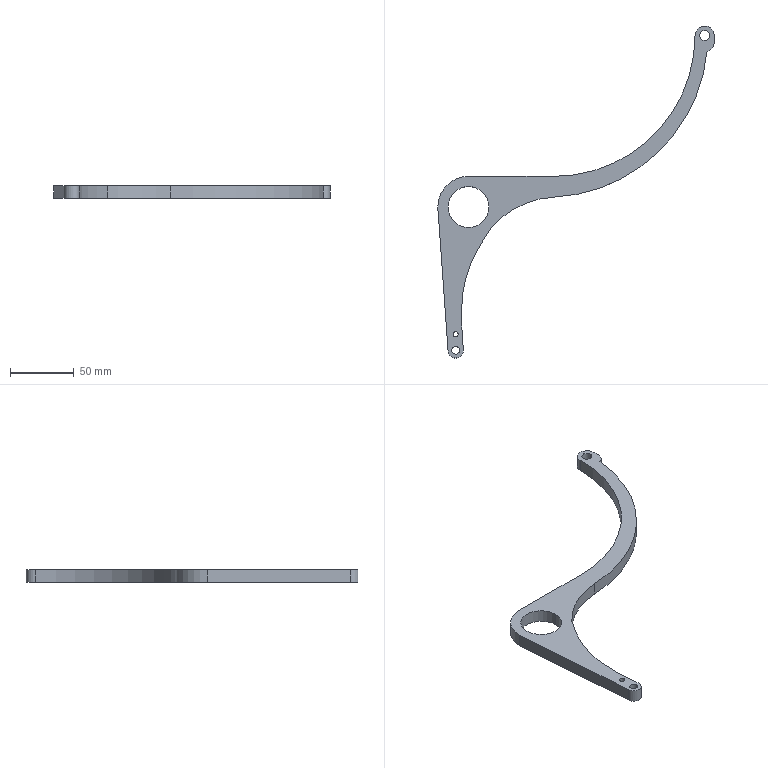Part | SolidWorks | features Extrusion 1 | 1 solid | 21 faces | box 216 x 259.5 x 10 mm | volume 61129 mm3 | cylinder 15 | plane 5 | spline 1 | commonest cylinder face diameters 4 x2 6 x2 7.838 x2 32 x2 12 x1 15 x1
STEP:
#1=CARTESIAN_POINT('',(-2.,12.5,10.));
#2=VERTEX_POINT('',#1);
#3=CARTESIAN_POINT('',(2.,12.5,10.));
#4=VERTEX_POINT('',#3);
#5=CARTESIAN_POINT('',(0.,12.5,10.));
#6=DIRECTION('',(0.,0.,1.));
#7=DIRECTION('',(1.,0.,0.));
#8=AXIS2_PLACEMENT_3D('',#5,#6,#7);
#9=CIRCLE('',#8,2.);
#10=EDGE_CURVE('',#2,#4,#9,.T.);
#11=ORIENTED_EDGE('',*,*,#10,.T.);
#12=CARTESIAN_POINT('',(2.,12.5,0.));
#13=VERTEX_POINT('',#12);
#14=CARTESIAN_POINT('',(2.,12.5,10.));
#15=DIRECTION('',(0.,0.,-1.));
#16=VECTOR('',#15,1000.);
#17=LINE('',#14,#16);
#18=EDGE_CURVE('',#4,#13,#17,.T.);
#19=ORIENTED_EDGE('',*,*,#18,.T.);
#20=CARTESIAN_POINT('',(-2.,12.5,0.));
#21=VERTEX_POINT('',#20);
#22=CARTESIAN_POINT('',(0.,12.5,0.));
#23=DIRECTION('',(0.,0.,1.));
#24=DIRECTION('',(1.,0.,0.));
#25=AXIS2_PLACEMENT_3D('',#22,#23,#24);
#26=CIRCLE('',#25,2.);
#27=EDGE_CURVE('',#21,#13,#26,.T.);
#28=ORIENTED_EDGE('',*,*,#27,.F.);
#29=CARTESIAN_POINT('',(-2.,12.5,10.));
#30=DIRECTION('',(0.,0.,-1.));
#31=VECTOR('',#30,1000.);
#32=LINE('',#29,#31);
#33=EDGE_CURVE('',#2,#21,#32,.T.);
#34=ORIENTED_EDGE('',*,*,#33,.F.);
#35=EDGE_LOOP('',(#11,#19,#28,#34));
#36=FACE_OUTER_BOUND('',#35,.T.);
#37=CARTESIAN_POINT('',(0.,12.5,10.));
#38=DIRECTION('',(0.,0.,-1.));
#39=DIRECTION('',(-1.,0.,0.));
#40=AXIS2_PLACEMENT_3D('',#37,#38,#39);
#41=CYLINDRICAL_SURFACE('',#40,2.);
#42=ADVANCED_FACE('',(#36),#41,.F.);
#43=CARTESIAN_POINT('',(190.581,246.,10.));
#44=VERTEX_POINT('',#43);
#45=CARTESIAN_POINT('',(198.419,246.,10.));
#46=VERTEX_POINT('',#45);
#47=CARTESIAN_POINT('',(194.5,246.,10.));
#48=DIRECTION('',(0.,0.,1.));
#49=DIRECTION('',(1.,0.,0.));
#50=AXIS2_PLACEMENT_3D('',#47,#48,#49);
#51=CIRCLE('',#50,3.919);
#52=EDGE_CURVE('',#44,#46,#51,.T.);
#53=ORIENTED_EDGE('',*,*,#52,.T.);
#54=CARTESIAN_POINT('',(198.419,246.,0.));
#55=VERTEX_POINT('',#54);
#56=CARTESIAN_POINT('',(198.419,246.,10.));
#57=DIRECTION('',(0.,0.,-1.));
#58=VECTOR('',#57,1000.);
#59=LINE('',#56,#58);
#60=EDGE_CURVE('',#46,#55,#59,.T.);
#61=ORIENTED_EDGE('',*,*,#60,.T.);
#62=CARTESIAN_POINT('',(190.581,246.,0.));
#63=VERTEX_POINT('',#62);
#64=CARTESIAN_POINT('',(194.5,246.,0.));
#65=DIRECTION('',(0.,0.,1.));
#66=DIRECTION('',(1.,0.,0.));
#67=AXIS2_PLACEMENT_3D('',#64,#65,#66);
#68=CIRCLE('',#67,3.919);
#69=EDGE_CURVE('',#63,#55,#68,.T.);
#70=ORIENTED_EDGE('',*,*,#69,.F.);
#71=CARTESIAN_POINT('',(190.581,246.,10.));
#72=DIRECTION('',(0.,0.,-1.));
#73=VECTOR('',#72,1000.);
#74=LINE('',#71,#73);
#75=EDGE_CURVE('',#44,#63,#74,.T.);
#76=ORIENTED_EDGE('',*,*,#75,.F.);
#77=EDGE_LOOP('',(#53,#61,#70,#76));
#78=FACE_OUTER_BOUND('',#77,.T.);
#79=CARTESIAN_POINT('',(194.5,246.,10.));
#80=DIRECTION('',(0.,0.,-1.));
#81=DIRECTION('',(-1.,0.,0.));
#82=AXIS2_PLACEMENT_3D('',#79,#80,#81);
#83=CYLINDRICAL_SURFACE('',#82,3.919);
#84=ADVANCED_FACE('',(#78),#83,.F.);
#85=CARTESIAN_POINT('',(-6.,112.,10.));
#86=VERTEX_POINT('',#85);
#87=CARTESIAN_POINT('',(26.,112.,10.));
#88=VERTEX_POINT('',#87);
#89=CARTESIAN_POINT('',(10.,112.,10.));
#90=DIRECTION('',(0.,0.,1.));
#91=DIRECTION('',(1.,0.,0.));
#92=AXIS2_PLACEMENT_3D('',#89,#90,#91);
#93=CIRCLE('',#92,16.);
#94=EDGE_CURVE('',#86,#88,#93,.T.);
#95=ORIENTED_EDGE('',*,*,#94,.T.);
#96=CARTESIAN_POINT('',(26.,112.,0.));
#97=VERTEX_POINT('',#96);
#98=CARTESIAN_POINT('',(26.,112.,10.));
#99=DIRECTION('',(0.,0.,-1.));
#100=VECTOR('',#99,1000.);
#101=LINE('',#98,#100);
#102=EDGE_CURVE('',#88,#97,#101,.T.);
#103=ORIENTED_EDGE('',*,*,#102,.T.);
#104=CARTESIAN_POINT('',(-6.,112.,0.));
#105=VERTEX_POINT('',#104);
#106=CARTESIAN_POINT('',(10.,112.,0.));
#107=DIRECTION('',(0.,0.,1.));
#108=DIRECTION('',(1.,0.,0.));
#109=AXIS2_PLACEMENT_3D('',#106,#107,#108);
#110=CIRCLE('',#109,16.);
#111=EDGE_CURVE('',#105,#97,#110,.T.);
#112=ORIENTED_EDGE('',*,*,#111,.F.);
#113=CARTESIAN_POINT('',(-6.,112.,10.));
#114=DIRECTION('',(0.,0.,-1.));
#115=VECTOR('',#114,1000.);
#116=LINE('',#113,#115);
#117=EDGE_CURVE('',#86,#105,#116,.T.);
#118=ORIENTED_EDGE('',*,*,#117,.F.);
#119=EDGE_LOOP('',(#95,#103,#112,#118));
#120=FACE_OUTER_BOUND('',#119,.T.);
#121=CARTESIAN_POINT('',(10.,112.,10.));
#122=DIRECTION('',(0.,0.,-1.));
#123=DIRECTION('',(-1.,0.,0.));
#124=AXIS2_PLACEMENT_3D('',#121,#122,#123);
#125=CYLINDRICAL_SURFACE('',#124,16.);
#126=ADVANCED_FACE('',(#120),#125,.F.);
#127=CARTESIAN_POINT('',(-3.,0.,10.));
#128=VERTEX_POINT('',#127);
#129=CARTESIAN_POINT('',(3.,0.,10.));
#130=VERTEX_POINT('',#129);
#131=CARTESIAN_POINT('',(0.,0.,10.));
#132=DIRECTION('',(0.,0.,1.));
#133=DIRECTION('',(1.,0.,0.));
#134=AXIS2_PLACEMENT_3D('',#131,#132,#133);
#135=CIRCLE('',#134,3.);
#136=EDGE_CURVE('',#128,#130,#135,.T.);
#137=ORIENTED_EDGE('',*,*,#136,.T.);
#138=CARTESIAN_POINT('',(3.,0.,0.));
#139=VERTEX_POINT('',#138);
#140=CARTESIAN_POINT('',(3.,0.,10.));
#141=DIRECTION('',(0.,0.,-1.));
#142=VECTOR('',#141,1000.);
#143=LINE('',#140,#142);
#144=EDGE_CURVE('',#130,#139,#143,.T.);
#145=ORIENTED_EDGE('',*,*,#144,.T.);
#146=CARTESIAN_POINT('',(-3.,0.,0.));
#147=VERTEX_POINT('',#146);
#148=CARTESIAN_POINT('',(0.,0.,0.));
#149=DIRECTION('',(0.,0.,1.));
#150=DIRECTION('',(1.,0.,0.));
#151=AXIS2_PLACEMENT_3D('',#148,#149,#150);
#152=CIRCLE('',#151,3.);
#153=EDGE_CURVE('',#147,#139,#152,.T.);
#154=ORIENTED_EDGE('',*,*,#153,.F.);
#155=CARTESIAN_POINT('',(-3.,0.,10.));
#156=DIRECTION('',(0.,0.,-1.));
#157=VECTOR('',#156,1000.);
#158=LINE('',#155,#157);
#159=EDGE_CURVE('',#128,#147,#158,.T.);
#160=ORIENTED_EDGE('',*,*,#159,.F.);
#161=EDGE_LOOP('',(#137,#145,#154,#160));
#162=FACE_OUTER_BOUND('',#161,.T.);
#163=CARTESIAN_POINT('',(0.,0.,10.));
#164=DIRECTION('',(0.,0.,-1.));
#165=DIRECTION('',(-1.,0.,0.));
#166=AXIS2_PLACEMENT_3D('',#163,#164,#165);
#167=CYLINDRICAL_SURFACE('',#166,3.);
#168=ADVANCED_FACE('',(#162),#167,.F.);
#169=ORIENTED_EDGE('',*,*,#52,.F.);
#170=CARTESIAN_POINT('',(194.5,246.,10.));
#171=DIRECTION('',(0.,0.,1.));
#172=DIRECTION('',(1.,0.,0.));
#173=AXIS2_PLACEMENT_3D('',#170,#171,#172);
#174=CIRCLE('',#173,3.919);
#175=EDGE_CURVE('',#46,#44,#174,.T.);
#176=ORIENTED_EDGE('',*,*,#175,.F.);
#177=EDGE_LOOP('',(#169,#176));
#178=FACE_BOUND('',#177,.T.);
#179=ORIENTED_EDGE('',*,*,#136,.F.);
#180=CARTESIAN_POINT('',(0.,0.,10.));
#181=DIRECTION('',(0.,0.,1.));
#182=DIRECTION('',(1.,0.,0.));
#183=AXIS2_PLACEMENT_3D('',#180,#181,#182);
#184=CIRCLE('',#183,3.);
#185=EDGE_CURVE('',#130,#128,#184,.T.);
#186=ORIENTED_EDGE('',*,*,#185,.F.);
#187=EDGE_LOOP('',(#179,#186));
#188=FACE_BOUND('',#187,.T.);
#189=CARTESIAN_POINT('',(10.,136.,10.));
#190=VERTEX_POINT('',#189);
#191=CARTESIAN_POINT('',(-14.,112.,10.));
#192=VERTEX_POINT('',#191);
#193=CARTESIAN_POINT('',(10.,112.,10.));
#194=DIRECTION('',(0.,0.,1.));
#195=DIRECTION('',(1.,0.,0.));
#196=AXIS2_PLACEMENT_3D('',#193,#194,#195);
#197=CIRCLE('',#196,24.);
#198=EDGE_CURVE('',#190,#192,#197,.T.);
#199=ORIENTED_EDGE('',*,*,#198,.T.);
#200=CARTESIAN_POINT('',(-6.,0.,10.));
#201=VERTEX_POINT('',#200);
#202=CARTESIAN_POINT('',(-14.,112.,10.));
#203=DIRECTION('',(0.07125,-0.9975,0.));
#204=VECTOR('',#203,1000.);
#205=LINE('',#202,#204);
#206=EDGE_CURVE('',#192,#201,#205,.T.);
#207=ORIENTED_EDGE('',*,*,#206,.T.);
#208=CARTESIAN_POINT('',(6.,0.,10.));
#209=VERTEX_POINT('',#208);
#210=CARTESIAN_POINT('',(0.,0.,10.));
#211=DIRECTION('',(0.,0.,1.));
#212=DIRECTION('',(1.,0.,0.));
#213=AXIS2_PLACEMENT_3D('',#210,#211,#212);
#214=CIRCLE('',#213,6.);
#215=EDGE_CURVE('',#201,#209,#214,.T.);
#216=ORIENTED_EDGE('',*,*,#215,.T.);
#217=CARTESIAN_POINT('',(28.005,96.131,10.));
#218=VERTEX_POINT('',#217);
#219=CARTESIAN_POINT('',(6.,0.,10.));
#220=CARTESIAN_POINT('',(1.589,45.681,10.));
#221=CARTESIAN_POINT('',(5.604,63.643,10.));
#222=CARTESIAN_POINT('',(28.005,96.131,10.));
#223=B_SPLINE_CURVE_WITH_KNOTS('',3,(#219,#220,#221,#222),.UNSPECIFIED.,.F.,.F.,(4,4),(0.,0.7882),.UNSPECIFIED.);
#224=EDGE_CURVE('',#209,#218,#223,.T.);
#225=ORIENTED_EDGE('',*,*,#224,.T.);
#226=CARTESIAN_POINT('',(77.,119.767,10.));
#227=VERTEX_POINT('',#226);
#228=CARTESIAN_POINT('',(80.543,49.825,10.));
#229=DIRECTION('',(0.,0.,-1.));
#230=DIRECTION('',(1.,0.,0.));
#231=AXIS2_PLACEMENT_3D('',#228,#229,#230);
#232=CIRCLE('',#231,70.032);
#233=EDGE_CURVE('',#218,#227,#232,.T.);
#234=ORIENTED_EDGE('',*,*,#233,.T.);
#235=CARTESIAN_POINT('',(196.38,233.495,10.));
#236=VERTEX_POINT('',#235);
#237=CARTESIAN_POINT('',(70.606,246.,10.));
#238=DIRECTION('',(0.,0.,1.));
#239=DIRECTION('',(1.,0.,0.));
#240=AXIS2_PLACEMENT_3D('',#237,#238,#239);
#241=CIRCLE('',#240,126.394);
#242=EDGE_CURVE('',#227,#236,#241,.T.);
#243=ORIENTED_EDGE('',*,*,#242,.T.);
#244=CARTESIAN_POINT('',(202.,241.,10.));
#245=VERTEX_POINT('',#244);
#246=CARTESIAN_POINT('',(194.179,241.,10.));
#247=DIRECTION('',(0.,0.,1.));
#248=DIRECTION('',(1.,0.,0.));
#249=AXIS2_PLACEMENT_3D('',#246,#247,#248);
#250=CIRCLE('',#249,7.821);
#251=EDGE_CURVE('',#236,#245,#250,.T.);
#252=ORIENTED_EDGE('',*,*,#251,.T.);
#253=CARTESIAN_POINT('',(202.,246.,10.));
#254=VERTEX_POINT('',#253);
#255=CARTESIAN_POINT('',(202.,246.,10.));
#256=DIRECTION('',(0.,1.,0.));
#257=VECTOR('',#256,1000.);
#258=LINE('',#255,#257);
#259=EDGE_CURVE('',#245,#254,#258,.T.);
#260=ORIENTED_EDGE('',*,*,#259,.T.);
#261=CARTESIAN_POINT('',(187.,246.,10.));
#262=VERTEX_POINT('',#261);
#263=CARTESIAN_POINT('',(194.5,246.,10.));
#264=DIRECTION('',(0.,0.,1.));
#265=DIRECTION('',(1.,0.,0.));
#266=AXIS2_PLACEMENT_3D('',#263,#264,#265);
#267=CIRCLE('',#266,7.5);
#268=EDGE_CURVE('',#254,#262,#267,.T.);
#269=ORIENTED_EDGE('',*,*,#268,.T.);
#270=CARTESIAN_POINT('',(77.,136.,10.));
#271=VERTEX_POINT('',#270);
#272=CARTESIAN_POINT('',(77.,246.,10.));
#273=DIRECTION('',(0.,0.,-1.));
#274=DIRECTION('',(1.,0.,0.));
#275=AXIS2_PLACEMENT_3D('',#272,#273,#274);
#276=CIRCLE('',#275,110.);
#277=EDGE_CURVE('',#262,#271,#276,.T.);
#278=ORIENTED_EDGE('',*,*,#277,.T.);
#279=CARTESIAN_POINT('',(10.,136.,10.));
#280=DIRECTION('',(-1.,0.,0.));
#281=VECTOR('',#280,1000.);
#282=LINE('',#279,#281);
#283=EDGE_CURVE('',#271,#190,#282,.T.);
#284=ORIENTED_EDGE('',*,*,#283,.T.);
#285=EDGE_LOOP('',(#199,#207,#216,#225,#234,#243,#252,#260,#269,#278,#284));
#286=FACE_OUTER_BOUND('',#285,.T.);
#287=ORIENTED_EDGE('',*,*,#94,.F.);
#288=CARTESIAN_POINT('',(10.,112.,10.));
#289=DIRECTION('',(0.,0.,1.));
#290=DIRECTION('',(1.,0.,0.));
#291=AXIS2_PLACEMENT_3D('',#288,#289,#290);
#292=CIRCLE('',#291,16.);
#293=EDGE_CURVE('',#88,#86,#292,.T.);
#294=ORIENTED_EDGE('',*,*,#293,.F.);
#295=EDGE_LOOP('',(#287,#294));
#296=FACE_BOUND('',#295,.T.);
#297=ORIENTED_EDGE('',*,*,#10,.F.);
#298=CARTESIAN_POINT('',(0.,12.5,10.));
#299=DIRECTION('',(0.,0.,1.));
#300=DIRECTION('',(1.,0.,0.));
#301=AXIS2_PLACEMENT_3D('',#298,#299,#300);
#302=CIRCLE('',#301,2.);
#303=EDGE_CURVE('',#4,#2,#302,.T.);
#304=ORIENTED_EDGE('',*,*,#303,.F.);
#305=EDGE_LOOP('',(#297,#304));
#306=FACE_BOUND('',#305,.T.);
#307=CARTESIAN_POINT('',(10.,112.,10.));
#308=DIRECTION('',(0.,0.,1.));
#309=DIRECTION('',(1.,0.,0.));
#310=AXIS2_PLACEMENT_3D('',#307,#308,#309);
#311=PLANE('',#310);
#312=ADVANCED_FACE('',(#178,#188,#286,#296,#306),#311,.T.);
#313=CARTESIAN_POINT('',(10.,136.,0.));
#314=VERTEX_POINT('',#313);
#315=CARTESIAN_POINT('',(-14.,112.,0.));
#316=VERTEX_POINT('',#315);
#317=CARTESIAN_POINT('',(10.,112.,0.));
#318=DIRECTION('',(0.,0.,1.));
#319=DIRECTION('',(1.,0.,0.));
#320=AXIS2_PLACEMENT_3D('',#317,#318,#319);
#321=CIRCLE('',#320,24.);
#322=EDGE_CURVE('',#314,#316,#321,.T.);
#323=ORIENTED_EDGE('',*,*,#322,.F.);
#324=CARTESIAN_POINT('',(77.,136.,0.));
#325=VERTEX_POINT('',#324);
#326=CARTESIAN_POINT('',(10.,136.,0.));
#327=DIRECTION('',(-1.,0.,0.));
#328=VECTOR('',#327,1000.);
#329=LINE('',#326,#328);
#330=EDGE_CURVE('',#325,#314,#329,.T.);
#331=ORIENTED_EDGE('',*,*,#330,.F.);
#332=CARTESIAN_POINT('',(187.,246.,0.));
#333=VERTEX_POINT('',#332);
#334=CARTESIAN_POINT('',(77.,246.,0.));
#335=DIRECTION('',(0.,0.,-1.));
#336=DIRECTION('',(1.,0.,0.));
#337=AXIS2_PLACEMENT_3D('',#334,#335,#336);
#338=CIRCLE('',#337,110.);
#339=EDGE_CURVE('',#333,#325,#338,.T.);
#340=ORIENTED_EDGE('',*,*,#339,.F.);
#341=CARTESIAN_POINT('',(202.,246.,0.));
#342=VERTEX_POINT('',#341);
#343=CARTESIAN_POINT('',(194.5,246.,0.));
#344=DIRECTION('',(0.,0.,1.));
#345=DIRECTION('',(1.,0.,0.));
#346=AXIS2_PLACEMENT_3D('',#343,#344,#345);
#347=CIRCLE('',#346,7.5);
#348=EDGE_CURVE('',#342,#333,#347,.T.);
#349=ORIENTED_EDGE('',*,*,#348,.F.);
#350=CARTESIAN_POINT('',(202.,241.,0.));
#351=VERTEX_POINT('',#350);
#352=CARTESIAN_POINT('',(202.,246.,0.));
#353=DIRECTION('',(0.,1.,0.));
#354=VECTOR('',#353,1000.);
#355=LINE('',#352,#354);
#356=EDGE_CURVE('',#351,#342,#355,.T.);
#357=ORIENTED_EDGE('',*,*,#356,.F.);
#358=CARTESIAN_POINT('',(196.38,233.495,0.));
#359=VERTEX_POINT('',#358);
#360=CARTESIAN_POINT('',(194.179,241.,0.));
#361=DIRECTION('',(0.,0.,1.));
#362=DIRECTION('',(1.,0.,0.));
#363=AXIS2_PLACEMENT_3D('',#360,#361,#362);
#364=CIRCLE('',#363,7.821);
#365=EDGE_CURVE('',#359,#351,#364,.T.);
#366=ORIENTED_EDGE('',*,*,#365,.F.);
#367=CARTESIAN_POINT('',(77.,119.767,0.));
#368=VERTEX_POINT('',#367);
#369=CARTESIAN_POINT('',(70.606,246.,0.));
#370=DIRECTION('',(0.,0.,1.));
#371=DIRECTION('',(1.,0.,0.));
#372=AXIS2_PLACEMENT_3D('',#369,#370,#371);
#373=CIRCLE('',#372,126.394);
#374=EDGE_CURVE('',#368,#359,#373,.T.);
#375=ORIENTED_EDGE('',*,*,#374,.F.);
#376=CARTESIAN_POINT('',(28.005,96.131,0.));
#377=VERTEX_POINT('',#376);
#378=CARTESIAN_POINT('',(80.543,49.825,0.));
#379=DIRECTION('',(0.,0.,-1.));
#380=DIRECTION('',(1.,0.,0.));
#381=AXIS2_PLACEMENT_3D('',#378,#379,#380);
#382=CIRCLE('',#381,70.032);
#383=EDGE_CURVE('',#377,#368,#382,.T.);
#384=ORIENTED_EDGE('',*,*,#383,.F.);
#385=CARTESIAN_POINT('',(6.,0.,0.));
#386=VERTEX_POINT('',#385);
#387=CARTESIAN_POINT('',(6.,0.,0.));
#388=CARTESIAN_POINT('',(1.589,45.681,0.));
#389=CARTESIAN_POINT('',(5.604,63.643,0.));
#390=CARTESIAN_POINT('',(28.005,96.131,0.));
#391=B_SPLINE_CURVE_WITH_KNOTS('',3,(#387,#388,#389,#390),.UNSPECIFIED.,.F.,.F.,(4,4),(0.,0.7882),.UNSPECIFIED.);
#392=EDGE_CURVE('',#386,#377,#391,.T.);
#393=ORIENTED_EDGE('',*,*,#392,.F.);
#394=CARTESIAN_POINT('',(-6.,0.,0.));
#395=VERTEX_POINT('',#394);
#396=CARTESIAN_POINT('',(0.,0.,0.));
#397=DIRECTION('',(0.,0.,1.));
#398=DIRECTION('',(1.,0.,0.));
#399=AXIS2_PLACEMENT_3D('',#396,#397,#398);
#400=CIRCLE('',#399,6.);
#401=EDGE_CURVE('',#395,#386,#400,.T.);
#402=ORIENTED_EDGE('',*,*,#401,.F.);
#403=CARTESIAN_POINT('',(-14.,112.,0.));
#404=DIRECTION('',(0.07125,-0.9975,0.));
#405=VECTOR('',#404,1000.);
#406=LINE('',#403,#405);
#407=EDGE_CURVE('',#316,#395,#406,.T.);
#408=ORIENTED_EDGE('',*,*,#407,.F.);
#409=EDGE_LOOP('',(#323,#331,#340,#349,#357,#366,#375,#384,#393,#402,#408));
#410=FACE_OUTER_BOUND('',#409,.T.);
#411=ORIENTED_EDGE('',*,*,#153,.T.);
#412=CARTESIAN_POINT('',(0.,0.,0.));
#413=DIRECTION('',(0.,0.,1.));
#414=DIRECTION('',(1.,0.,0.));
#415=AXIS2_PLACEMENT_3D('',#412,#413,#414);
#416=CIRCLE('',#415,3.);
#417=EDGE_CURVE('',#139,#147,#416,.T.);
#418=ORIENTED_EDGE('',*,*,#417,.T.);
#419=EDGE_LOOP('',(#411,#418));
#420=FACE_BOUND('',#419,.T.);
#421=ORIENTED_EDGE('',*,*,#111,.T.);
#422=CARTESIAN_POINT('',(10.,112.,0.));
#423=DIRECTION('',(0.,0.,1.));
#424=DIRECTION('',(1.,0.,0.));
#425=AXIS2_PLACEMENT_3D('',#422,#423,#424);
#426=CIRCLE('',#425,16.);
#427=EDGE_CURVE('',#97,#105,#426,.T.);
#428=ORIENTED_EDGE('',*,*,#427,.T.);
#429=EDGE_LOOP('',(#421,#428));
#430=FACE_BOUND('',#429,.T.);
#431=ORIENTED_EDGE('',*,*,#69,.T.);
#432=CARTESIAN_POINT('',(194.5,246.,0.));
#433=DIRECTION('',(0.,0.,1.));
#434=DIRECTION('',(1.,0.,0.));
#435=AXIS2_PLACEMENT_3D('',#432,#433,#434);
#436=CIRCLE('',#435,3.919);
#437=EDGE_CURVE('',#55,#63,#436,.T.);
#438=ORIENTED_EDGE('',*,*,#437,.T.);
#439=EDGE_LOOP('',(#431,#438));
#440=FACE_BOUND('',#439,.T.);
#441=ORIENTED_EDGE('',*,*,#27,.T.);
#442=CARTESIAN_POINT('',(0.,12.5,0.));
#443=DIRECTION('',(0.,0.,1.));
#444=DIRECTION('',(1.,0.,0.));
#445=AXIS2_PLACEMENT_3D('',#442,#443,#444);
#446=CIRCLE('',#445,2.);
#447=EDGE_CURVE('',#13,#21,#446,.T.);
#448=ORIENTED_EDGE('',*,*,#447,.T.);
#449=EDGE_LOOP('',(#441,#448));
#450=FACE_BOUND('',#449,.T.);
#451=CARTESIAN_POINT('',(10.,112.,0.));
#452=DIRECTION('',(0.,0.,1.));
#453=DIRECTION('',(1.,0.,0.));
#454=AXIS2_PLACEMENT_3D('',#451,#452,#453);
#455=PLANE('',#454);
#456=ADVANCED_FACE('',(#410,#420,#430,#440,#450),#455,.F.);
#457=ORIENTED_EDGE('',*,*,#322,.T.);
#458=CARTESIAN_POINT('',(-14.,112.,10.));
#459=DIRECTION('',(0.,0.,-1.));
#460=VECTOR('',#459,1000.);
#461=LINE('',#458,#460);
#462=EDGE_CURVE('',#192,#316,#461,.T.);
#463=ORIENTED_EDGE('',*,*,#462,.F.);
#464=ORIENTED_EDGE('',*,*,#198,.F.);
#465=CARTESIAN_POINT('',(10.,136.,10.));
#466=DIRECTION('',(0.,0.,-1.));
#467=VECTOR('',#466,1000.);
#468=LINE('',#465,#467);
#469=EDGE_CURVE('',#190,#314,#468,.T.);
#470=ORIENTED_EDGE('',*,*,#469,.T.);
#471=EDGE_LOOP('',(#457,#463,#464,#470));
#472=FACE_OUTER_BOUND('',#471,.T.);
#473=CARTESIAN_POINT('',(10.,112.,10.));
#474=DIRECTION('',(0.,0.,-1.));
#475=DIRECTION('',(-1.,0.,0.));
#476=AXIS2_PLACEMENT_3D('',#473,#474,#475);
#477=CYLINDRICAL_SURFACE('',#476,24.);
#478=ADVANCED_FACE('',(#472),#477,.T.);
#479=ORIENTED_EDGE('',*,*,#407,.T.);
#480=CARTESIAN_POINT('',(-6.,0.,10.));
#481=DIRECTION('',(0.,0.,-1.));
#482=VECTOR('',#481,1000.);
#483=LINE('',#480,#482);
#484=EDGE_CURVE('',#201,#395,#483,.T.);
#485=ORIENTED_EDGE('',*,*,#484,.F.);
#486=ORIENTED_EDGE('',*,*,#206,.F.);
#487=ORIENTED_EDGE('',*,*,#462,.T.);
#488=EDGE_LOOP('',(#479,#485,#486,#487));
#489=FACE_OUTER_BOUND('',#488,.T.);
#490=CARTESIAN_POINT('',(-14.,112.,10.));
#491=DIRECTION('',(0.9975,0.07125,0.));
#492=DIRECTION('',(-0.07125,0.9975,0.));
#493=AXIS2_PLACEMENT_3D('',#490,#491,#492);
#494=PLANE('',#493);
#495=ADVANCED_FACE('',(#489),#494,.F.);
#496=ORIENTED_EDGE('',*,*,#401,.T.);
#497=CARTESIAN_POINT('',(6.,0.,10.));
#498=DIRECTION('',(0.,0.,-1.));
#499=VECTOR('',#498,1000.);
#500=LINE('',#497,#499);
#501=EDGE_CURVE('',#209,#386,#500,.T.);
#502=ORIENTED_EDGE('',*,*,#501,.F.);
#503=ORIENTED_EDGE('',*,*,#215,.F.);
#504=ORIENTED_EDGE('',*,*,#484,.T.);
#505=EDGE_LOOP('',(#496,#502,#503,#504));
#506=FACE_OUTER_BOUND('',#505,.T.);
#507=CARTESIAN_POINT('',(0.,0.,10.));
#508=DIRECTION('',(0.,0.,-1.));
#509=DIRECTION('',(-1.,0.,0.));
#510=AXIS2_PLACEMENT_3D('',#507,#508,#509);
#511=CYLINDRICAL_SURFACE('',#510,6.);
#512=ADVANCED_FACE('',(#506),#511,.T.);
#513=ORIENTED_EDGE('',*,*,#392,.T.);
#514=CARTESIAN_POINT('',(28.005,96.131,10.));
#515=DIRECTION('',(0.,0.,-1.));
#516=VECTOR('',#515,1000.);
#517=LINE('',#514,#516);
#518=EDGE_CURVE('',#218,#377,#517,.T.);
#519=ORIENTED_EDGE('',*,*,#518,.F.);
#520=ORIENTED_EDGE('',*,*,#224,.F.);
#521=ORIENTED_EDGE('',*,*,#501,.T.);
#522=EDGE_LOOP('',(#513,#519,#520,#521));
#523=FACE_OUTER_BOUND('',#522,.T.);
#524=CARTESIAN_POINT('',(6.,0.,10.));
#525=CARTESIAN_POINT('',(6.,0.,0.));
#526=CARTESIAN_POINT('',(1.589,45.681,10.));
#527=CARTESIAN_POINT('',(1.589,45.681,0.));
#528=CARTESIAN_POINT('',(5.604,63.643,10.));
#529=CARTESIAN_POINT('',(5.604,63.643,0.));
#530=CARTESIAN_POINT('',(28.005,96.131,10.));
#531=CARTESIAN_POINT('',(28.005,96.131,0.));
#532=B_SPLINE_SURFACE_WITH_KNOTS('',3,1,((#524,#525),(#526,#527),(#528,#529),(#530,#531)),.UNSPECIFIED.,.F.,.F.,.F.,(4,4),(2,2),(0.,0.7882),(0.,1.),.UNSPECIFIED.);
#533=ADVANCED_FACE('',(#523),#532,.F.);
#534=ORIENTED_EDGE('',*,*,#383,.T.);
#535=CARTESIAN_POINT('',(77.,119.767,10.));
#536=DIRECTION('',(0.,0.,-1.));
#537=VECTOR('',#536,1000.);
#538=LINE('',#535,#537);
#539=EDGE_CURVE('',#227,#368,#538,.T.);
#540=ORIENTED_EDGE('',*,*,#539,.F.);
#541=ORIENTED_EDGE('',*,*,#233,.F.);
#542=ORIENTED_EDGE('',*,*,#518,.T.);
#543=EDGE_LOOP('',(#534,#540,#541,#542));
#544=FACE_OUTER_BOUND('',#543,.T.);
#545=CARTESIAN_POINT('',(80.543,49.825,10.));
#546=DIRECTION('',(0.,0.,-1.));
#547=DIRECTION('',(-1.,0.,0.));
#548=AXIS2_PLACEMENT_3D('',#545,#546,#547);
#549=CYLINDRICAL_SURFACE('',#548,70.032);
#550=ADVANCED_FACE('',(#544),#549,.F.);
#551=ORIENTED_EDGE('',*,*,#374,.T.);
#552=CARTESIAN_POINT('',(196.38,233.495,10.));
#553=DIRECTION('',(0.,0.,-1.));
#554=VECTOR('',#553,1000.);
#555=LINE('',#552,#554);
#556=EDGE_CURVE('',#236,#359,#555,.T.);
#557=ORIENTED_EDGE('',*,*,#556,.F.);
#558=ORIENTED_EDGE('',*,*,#242,.F.);
#559=ORIENTED_EDGE('',*,*,#539,.T.);
#560=EDGE_LOOP('',(#551,#557,#558,#559));
#561=FACE_OUTER_BOUND('',#560,.T.);
#562=CARTESIAN_POINT('',(70.606,246.,10.));
#563=DIRECTION('',(0.,0.,-1.));
#564=DIRECTION('',(-1.,0.,0.));
#565=AXIS2_PLACEMENT_3D('',#562,#563,#564);
#566=CYLINDRICAL_SURFACE('',#565,126.394);
#567=ADVANCED_FACE('',(#561),#566,.T.);
#568=ORIENTED_EDGE('',*,*,#365,.T.);
#569=CARTESIAN_POINT('',(202.,241.,10.));
#570=DIRECTION('',(0.,0.,-1.));
#571=VECTOR('',#570,1000.);
#572=LINE('',#569,#571);
#573=EDGE_CURVE('',#245,#351,#572,.T.);
#574=ORIENTED_EDGE('',*,*,#573,.F.);
#575=ORIENTED_EDGE('',*,*,#251,.F.);
#576=ORIENTED_EDGE('',*,*,#556,.T.);
#577=EDGE_LOOP('',(#568,#574,#575,#576));
#578=FACE_OUTER_BOUND('',#577,.T.);
#579=CARTESIAN_POINT('',(194.179,241.,10.));
#580=DIRECTION('',(0.,0.,-1.));
#581=DIRECTION('',(-1.,0.,0.));
#582=AXIS2_PLACEMENT_3D('',#579,#580,#581);
#583=CYLINDRICAL_SURFACE('',#582,7.821);
#584=ADVANCED_FACE('',(#578),#583,.T.);
#585=ORIENTED_EDGE('',*,*,#356,.T.);
#586=CARTESIAN_POINT('',(202.,246.,10.));
#587=DIRECTION('',(0.,0.,-1.));
#588=VECTOR('',#587,1000.);
#589=LINE('',#586,#588);
#590=EDGE_CURVE('',#254,#342,#589,.T.);
#591=ORIENTED_EDGE('',*,*,#590,.F.);
#592=ORIENTED_EDGE('',*,*,#259,.F.);
#593=ORIENTED_EDGE('',*,*,#573,.T.);
#594=EDGE_LOOP('',(#585,#591,#592,#593));
#595=FACE_OUTER_BOUND('',#594,.T.);
#596=CARTESIAN_POINT('',(202.,246.,10.));
#597=DIRECTION('',(-1.,0.,0.));
#598=DIRECTION('',(0.,0.,1.));
#599=AXIS2_PLACEMENT_3D('',#596,#597,#598);
#600=PLANE('',#599);
#601=ADVANCED_FACE('',(#595),#600,.F.);
#602=ORIENTED_EDGE('',*,*,#348,.T.);
#603=CARTESIAN_POINT('',(187.,246.,10.));
#604=DIRECTION('',(0.,0.,-1.));
#605=VECTOR('',#604,1000.);
#606=LINE('',#603,#605);
#607=EDGE_CURVE('',#262,#333,#606,.T.);
#608=ORIENTED_EDGE('',*,*,#607,.F.);
#609=ORIENTED_EDGE('',*,*,#268,.F.);
#610=ORIENTED_EDGE('',*,*,#590,.T.);
#611=EDGE_LOOP('',(#602,#608,#609,#610));
#612=FACE_OUTER_BOUND('',#611,.T.);
#613=CARTESIAN_POINT('',(194.5,246.,10.));
#614=DIRECTION('',(0.,0.,-1.));
#615=DIRECTION('',(-1.,0.,0.));
#616=AXIS2_PLACEMENT_3D('',#613,#614,#615);
#617=CYLINDRICAL_SURFACE('',#616,7.5);
#618=ADVANCED_FACE('',(#612),#617,.T.);
#619=ORIENTED_EDGE('',*,*,#339,.T.);
#620=CARTESIAN_POINT('',(77.,136.,10.));
#621=DIRECTION('',(0.,0.,-1.));
#622=VECTOR('',#621,1000.);
#623=LINE('',#620,#622);
#624=EDGE_CURVE('',#271,#325,#623,.T.);
#625=ORIENTED_EDGE('',*,*,#624,.F.);
#626=ORIENTED_EDGE('',*,*,#277,.F.);
#627=ORIENTED_EDGE('',*,*,#607,.T.);
#628=EDGE_LOOP('',(#619,#625,#626,#627));
#629=FACE_OUTER_BOUND('',#628,.T.);
#630=CARTESIAN_POINT('',(77.,246.,10.));
#631=DIRECTION('',(0.,0.,-1.));
#632=DIRECTION('',(-1.,0.,0.));
#633=AXIS2_PLACEMENT_3D('',#630,#631,#632);
#634=CYLINDRICAL_SURFACE('',#633,110.);
#635=ADVANCED_FACE('',(#629),#634,.F.);
#636=ORIENTED_EDGE('',*,*,#330,.T.);
#637=ORIENTED_EDGE('',*,*,#469,.F.);
#638=ORIENTED_EDGE('',*,*,#283,.F.);
#639=ORIENTED_EDGE('',*,*,#624,.T.);
#640=EDGE_LOOP('',(#636,#637,#638,#639));
#641=FACE_OUTER_BOUND('',#640,.T.);
#642=CARTESIAN_POINT('',(10.,136.,10.));
#643=DIRECTION('',(0.,-1.,0.));
#644=DIRECTION('',(0.,0.,-1.));
#645=AXIS2_PLACEMENT_3D('',#642,#643,#644);
#646=PLANE('',#645);
#647=ADVANCED_FACE('',(#641),#646,.F.);
#648=ORIENTED_EDGE('',*,*,#144,.F.);
#649=ORIENTED_EDGE('',*,*,#185,.T.);
#650=ORIENTED_EDGE('',*,*,#159,.T.);
#651=ORIENTED_EDGE('',*,*,#417,.F.);
#652=EDGE_LOOP('',(#648,#649,#650,#651));
#653=FACE_OUTER_BOUND('',#652,.T.);
#654=CARTESIAN_POINT('',(0.,0.,10.));
#655=DIRECTION('',(0.,0.,-1.));
#656=DIRECTION('',(-1.,0.,0.));
#657=AXIS2_PLACEMENT_3D('',#654,#655,#656);
#658=CYLINDRICAL_SURFACE('',#657,3.);
#659=ADVANCED_FACE('',(#653),#658,.F.);
#660=ORIENTED_EDGE('',*,*,#102,.F.);
#661=ORIENTED_EDGE('',*,*,#293,.T.);
#662=ORIENTED_EDGE('',*,*,#117,.T.);
#663=ORIENTED_EDGE('',*,*,#427,.F.);
#664=EDGE_LOOP('',(#660,#661,#662,#663));
#665=FACE_OUTER_BOUND('',#664,.T.);
#666=CARTESIAN_POINT('',(10.,112.,10.));
#667=DIRECTION('',(0.,0.,-1.));
#668=DIRECTION('',(-1.,0.,0.));
#669=AXIS2_PLACEMENT_3D('',#666,#667,#668);
#670=CYLINDRICAL_SURFACE('',#669,16.);
#671=ADVANCED_FACE('',(#665),#670,.F.);
#672=ORIENTED_EDGE('',*,*,#60,.F.);
#673=ORIENTED_EDGE('',*,*,#175,.T.);
#674=ORIENTED_EDGE('',*,*,#75,.T.);
#675=ORIENTED_EDGE('',*,*,#437,.F.);
#676=EDGE_LOOP('',(#672,#673,#674,#675));
#677=FACE_OUTER_BOUND('',#676,.T.);
#678=CARTESIAN_POINT('',(194.5,246.,10.));
#679=DIRECTION('',(0.,0.,-1.));
#680=DIRECTION('',(-1.,0.,0.));
#681=AXIS2_PLACEMENT_3D('',#678,#679,#680);
#682=CYLINDRICAL_SURFACE('',#681,3.919);
#683=ADVANCED_FACE('',(#677),#682,.F.);
#684=ORIENTED_EDGE('',*,*,#18,.F.);
#685=ORIENTED_EDGE('',*,*,#303,.T.);
#686=ORIENTED_EDGE('',*,*,#33,.T.);
#687=ORIENTED_EDGE('',*,*,#447,.F.);
#688=EDGE_LOOP('',(#684,#685,#686,#687));
#689=FACE_OUTER_BOUND('',#688,.T.);
#690=CARTESIAN_POINT('',(0.,12.5,10.));
#691=DIRECTION('',(0.,0.,-1.));
#692=DIRECTION('',(-1.,0.,0.));
#693=AXIS2_PLACEMENT_3D('',#690,#691,#692);
#694=CYLINDRICAL_SURFACE('',#693,2.);
#695=ADVANCED_FACE('',(#689),#694,.F.);
#696=CLOSED_SHELL('',(#42,#84,#126,#168,#312,#456,#478,#495,#512,#533,#550,#567,#584,#601,#618,#635,#647,#659,#671,#683,#695));
#697=MANIFOLD_SOLID_BREP('',#696);
#698=CARTESIAN_POINT('',(0.,0.,0.));
#699=DIRECTION('',(0.,0.,1.));
#700=DIRECTION('',(1.,0.,0.));
#701=AXIS2_PLACEMENT_3D('',#698,#699,#700);
#702=(LENGTH_UNIT()NAMED_UNIT(*)SI_UNIT(.MILLI.,.METRE.));
#703=UNCERTAINTY_MEASURE_WITH_UNIT(LENGTH_MEASURE(0.00001),#702,'','');
#704=(NAMED_UNIT(*)PLANE_ANGLE_UNIT()SI_UNIT($,.RADIAN.));
#705=(NAMED_UNIT(*)SI_UNIT($,.STERADIAN.)SOLID_ANGLE_UNIT());
#706=(GEOMETRIC_REPRESENTATION_CONTEXT(3)GLOBAL_UNCERTAINTY_ASSIGNED_CONTEXT((#703))GLOBAL_UNIT_ASSIGNED_CONTEXT((#702,#704,#705))REPRESENTATION_CONTEXT('',''));
#707=ADVANCED_BREP_SHAPE_REPRESENTATION('',(#697,#701),#706);